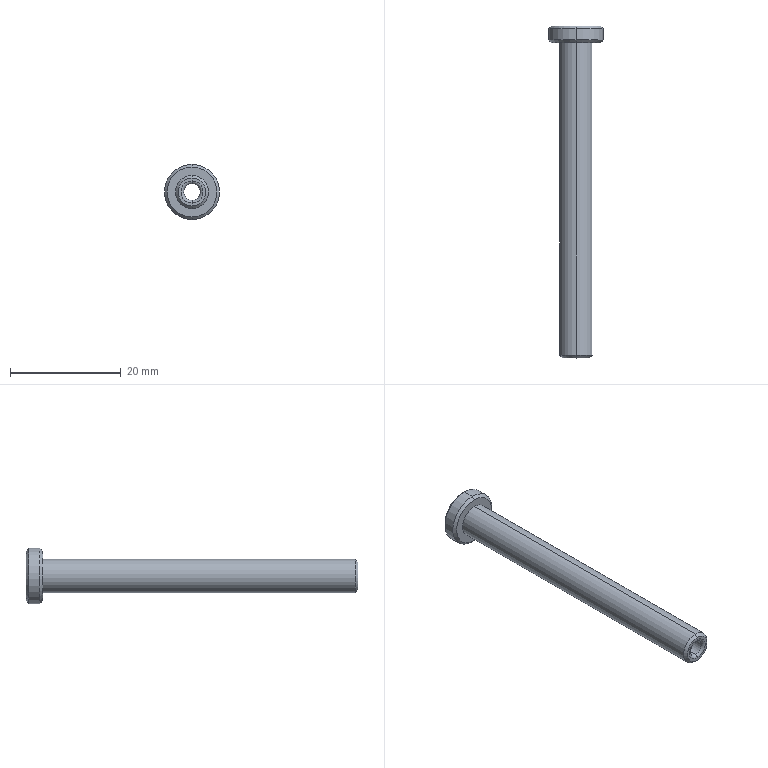Part | SolidWorks | features Chamfer 1, Extrusion 1, Fillet 1, ICE 1 | 1 solid | 19 faces | box 10 x 60 x 10 mm | volume 1412 mm3 | cone 6 | cylinder 6 | torus 4 | plane 3 | commonest cylinder face diameters 3 x2 6 x2 10 x2
STEP:
#1=CARTESIAN_POINT('',(0.,57.,-4.5));
#2=VERTEX_POINT('',#1);
#3=CARTESIAN_POINT('',(0.,57.,4.5));
#4=VERTEX_POINT('',#3);
#5=CARTESIAN_POINT('',(0.,57.,0.));
#6=DIRECTION('',(0.,-1.,0.));
#7=DIRECTION('',(0.,0.,1.));
#8=AXIS2_PLACEMENT_3D('',#5,#6,#7);
#9=CIRCLE('',#8,4.5);
#10=EDGE_CURVE('',#2,#4,#9,.T.);
#11=ORIENTED_EDGE('',*,*,#10,.F.);
#12=CARTESIAN_POINT('',(0.,57.5,-5.));
#13=VERTEX_POINT('',#12);
#14=CARTESIAN_POINT('',(0.,57.5,-5.));
#15=DIRECTION('',(0.,0.7071,-0.7071));
#16=VECTOR('',#15,1000.);
#17=LINE('',#14,#16);
#18=EDGE_CURVE('',#2,#13,#17,.T.);
#19=ORIENTED_EDGE('',*,*,#18,.T.);
#20=CARTESIAN_POINT('',(0.,57.5,5.));
#21=VERTEX_POINT('',#20);
#22=CARTESIAN_POINT('',(0.,57.5,0.));
#23=DIRECTION('',(0.,1.,0.));
#24=DIRECTION('',(0.,0.,1.));
#25=AXIS2_PLACEMENT_3D('',#22,#23,#24);
#26=CIRCLE('',#25,5.);
#27=EDGE_CURVE('',#21,#13,#26,.T.);
#28=ORIENTED_EDGE('',*,*,#27,.F.);
#29=CARTESIAN_POINT('',(0.,57.5,5.));
#30=DIRECTION('',(0.,0.7071,0.7071));
#31=VECTOR('',#30,1000.);
#32=LINE('',#29,#31);
#33=EDGE_CURVE('',#4,#21,#32,.T.);
#34=ORIENTED_EDGE('',*,*,#33,.F.);
#35=EDGE_LOOP('',(#11,#19,#28,#34));
#36=FACE_OUTER_BOUND('',#35,.T.);
#37=CARTESIAN_POINT('',(0.,57.5,0.));
#38=DIRECTION('',(0.,1.,0.));
#39=DIRECTION('',(0.,0.,1.));
#40=AXIS2_PLACEMENT_3D('',#37,#38,#39);
#41=CONICAL_SURFACE('',#40,5.,0.7854);
#42=ADVANCED_FACE('',(#36),#41,.T.);
#43=CARTESIAN_POINT('',(0.,0.,-2.5));
#44=VERTEX_POINT('',#43);
#45=CARTESIAN_POINT('',(0.,0.,2.5));
#46=VERTEX_POINT('',#45);
#47=CARTESIAN_POINT('',(0.,0.,0.));
#48=DIRECTION('',(0.,-1.,0.));
#49=DIRECTION('',(0.,0.,1.));
#50=AXIS2_PLACEMENT_3D('',#47,#48,#49);
#51=CIRCLE('',#50,2.5);
#52=EDGE_CURVE('',#44,#46,#51,.T.);
#53=ORIENTED_EDGE('',*,*,#52,.F.);
#54=CARTESIAN_POINT('',(0.,0.5,-3.));
#55=VERTEX_POINT('',#54);
#56=CARTESIAN_POINT('',(0.,0.5,-3.));
#57=DIRECTION('',(0.,0.7071,-0.7071));
#58=VECTOR('',#57,1000.);
#59=LINE('',#56,#58);
#60=EDGE_CURVE('',#44,#55,#59,.T.);
#61=ORIENTED_EDGE('',*,*,#60,.T.);
#62=CARTESIAN_POINT('',(0.,0.5,3.));
#63=VERTEX_POINT('',#62);
#64=CARTESIAN_POINT('',(0.,0.5,0.));
#65=DIRECTION('',(0.,1.,0.));
#66=DIRECTION('',(0.,0.,1.));
#67=AXIS2_PLACEMENT_3D('',#64,#65,#66);
#68=CIRCLE('',#67,3.);
#69=EDGE_CURVE('',#63,#55,#68,.T.);
#70=ORIENTED_EDGE('',*,*,#69,.F.);
#71=CARTESIAN_POINT('',(0.,0.5,3.));
#72=DIRECTION('',(0.,0.7071,0.7071));
#73=VECTOR('',#72,1000.);
#74=LINE('',#71,#73);
#75=EDGE_CURVE('',#46,#63,#74,.T.);
#76=ORIENTED_EDGE('',*,*,#75,.F.);
#77=EDGE_LOOP('',(#53,#61,#70,#76));
#78=FACE_OUTER_BOUND('',#77,.T.);
#79=CARTESIAN_POINT('',(0.,0.5,0.));
#80=DIRECTION('',(0.,1.,0.));
#81=DIRECTION('',(0.,0.,1.));
#82=AXIS2_PLACEMENT_3D('',#79,#80,#81);
#83=CONICAL_SURFACE('',#82,3.,0.7854);
#84=ADVANCED_FACE('',(#78),#83,.T.);
#85=CARTESIAN_POINT('',(0.,60.,4.5));
#86=VERTEX_POINT('',#85);
#87=CARTESIAN_POINT('',(0.,60.,-4.5));
#88=VERTEX_POINT('',#87);
#89=CARTESIAN_POINT('',(0.,60.,0.));
#90=DIRECTION('',(0.,1.,0.));
#91=DIRECTION('',(0.,0.,1.));
#92=AXIS2_PLACEMENT_3D('',#89,#90,#91);
#93=CIRCLE('',#92,4.5);
#94=EDGE_CURVE('',#86,#88,#93,.T.);
#95=ORIENTED_EDGE('',*,*,#94,.F.);
#96=CARTESIAN_POINT('',(0.,59.5,5.));
#97=VERTEX_POINT('',#96);
#98=CARTESIAN_POINT('',(0.,60.,4.5));
#99=DIRECTION('',(0.,-0.7071,0.7071));
#100=VECTOR('',#99,1000.);
#101=LINE('',#98,#100);
#102=EDGE_CURVE('',#86,#97,#101,.T.);
#103=ORIENTED_EDGE('',*,*,#102,.T.);
#104=CARTESIAN_POINT('',(0.,59.5,-5.));
#105=VERTEX_POINT('',#104);
#106=CARTESIAN_POINT('',(0.,59.5,0.));
#107=DIRECTION('',(0.,-1.,0.));
#108=DIRECTION('',(0.,0.,1.));
#109=AXIS2_PLACEMENT_3D('',#106,#107,#108);
#110=CIRCLE('',#109,5.);
#111=EDGE_CURVE('',#105,#97,#110,.T.);
#112=ORIENTED_EDGE('',*,*,#111,.F.);
#113=CARTESIAN_POINT('',(0.,60.,-4.5));
#114=DIRECTION('',(0.,-0.7071,-0.7071));
#115=VECTOR('',#114,1000.);
#116=LINE('',#113,#115);
#117=EDGE_CURVE('',#88,#105,#116,.T.);
#118=ORIENTED_EDGE('',*,*,#117,.F.);
#119=EDGE_LOOP('',(#95,#103,#112,#118));
#120=FACE_OUTER_BOUND('',#119,.T.);
#121=CARTESIAN_POINT('',(0.,60.,0.));
#122=DIRECTION('',(0.,-1.,0.));
#123=DIRECTION('',(0.,0.,-1.));
#124=AXIS2_PLACEMENT_3D('',#121,#122,#123);
#125=CONICAL_SURFACE('',#124,4.5,0.7854);
#126=ADVANCED_FACE('',(#120),#125,.T.);
#127=CARTESIAN_POINT('',(0.,0.5,-1.5));
#128=VERTEX_POINT('',#127);
#129=CARTESIAN_POINT('',(0.,0.5,1.5));
#130=VERTEX_POINT('',#129);
#131=CARTESIAN_POINT('',(0.,0.5,0.));
#132=DIRECTION('',(0.,-1.,0.));
#133=DIRECTION('',(0.,0.,1.));
#134=AXIS2_PLACEMENT_3D('',#131,#132,#133);
#135=CIRCLE('',#134,1.5);
#136=EDGE_CURVE('',#128,#130,#135,.T.);
#137=ORIENTED_EDGE('',*,*,#136,.F.);
#138=CARTESIAN_POINT('',(0.,0.,-2.));
#139=VERTEX_POINT('',#138);
#140=CARTESIAN_POINT('',(0.,0.5,-2.));
#141=DIRECTION('',(1.,0.,0.));
#142=DIRECTION('',(0.,0.,-1.));
#143=AXIS2_PLACEMENT_3D('',#140,#141,#142);
#144=CIRCLE('',#143,0.5);
#145=EDGE_CURVE('',#128,#139,#144,.T.);
#146=ORIENTED_EDGE('',*,*,#145,.T.);
#147=CARTESIAN_POINT('',(0.,0.,2.));
#148=VERTEX_POINT('',#147);
#149=CARTESIAN_POINT('',(0.,0.,0.));
#150=DIRECTION('',(0.,1.,0.));
#151=DIRECTION('',(0.,0.,1.));
#152=AXIS2_PLACEMENT_3D('',#149,#150,#151);
#153=CIRCLE('',#152,2.);
#154=EDGE_CURVE('',#148,#139,#153,.T.);
#155=ORIENTED_EDGE('',*,*,#154,.F.);
#156=CARTESIAN_POINT('',(0.,0.5,2.));
#157=DIRECTION('',(-1.,0.,0.));
#158=DIRECTION('',(0.,0.,1.));
#159=AXIS2_PLACEMENT_3D('',#156,#157,#158);
#160=CIRCLE('',#159,0.5);
#161=EDGE_CURVE('',#130,#148,#160,.T.);
#162=ORIENTED_EDGE('',*,*,#161,.F.);
#163=EDGE_LOOP('',(#137,#146,#155,#162));
#164=FACE_OUTER_BOUND('',#163,.T.);
#165=CARTESIAN_POINT('',(0.,0.5,0.));
#166=DIRECTION('',(0.,1.,0.));
#167=DIRECTION('',(0.,0.,1.));
#168=AXIS2_PLACEMENT_3D('',#165,#166,#167);
#169=TOROIDAL_SURFACE('',#168,2.,0.5);
#170=ADVANCED_FACE('',(#164),#169,.T.);
#171=CARTESIAN_POINT('',(0.,60.,-2.));
#172=VERTEX_POINT('',#171);
#173=CARTESIAN_POINT('',(0.,60.,2.));
#174=VERTEX_POINT('',#173);
#175=CARTESIAN_POINT('',(0.,60.,0.));
#176=DIRECTION('',(0.,-1.,0.));
#177=DIRECTION('',(0.,0.,1.));
#178=AXIS2_PLACEMENT_3D('',#175,#176,#177);
#179=CIRCLE('',#178,2.);
#180=EDGE_CURVE('',#172,#174,#179,.T.);
#181=ORIENTED_EDGE('',*,*,#180,.F.);
#182=CARTESIAN_POINT('',(0.,59.5,-1.5));
#183=VERTEX_POINT('',#182);
#184=CARTESIAN_POINT('',(0.,59.5,-2.));
#185=DIRECTION('',(1.,0.,0.));
#186=DIRECTION('',(0.,0.,-1.));
#187=AXIS2_PLACEMENT_3D('',#184,#185,#186);
#188=CIRCLE('',#187,0.5);
#189=EDGE_CURVE('',#172,#183,#188,.T.);
#190=ORIENTED_EDGE('',*,*,#189,.T.);
#191=CARTESIAN_POINT('',(0.,59.5,1.5));
#192=VERTEX_POINT('',#191);
#193=CARTESIAN_POINT('',(0.,59.5,0.));
#194=DIRECTION('',(0.,1.,0.));
#195=DIRECTION('',(0.,0.,1.));
#196=AXIS2_PLACEMENT_3D('',#193,#194,#195);
#197=CIRCLE('',#196,1.5);
#198=EDGE_CURVE('',#192,#183,#197,.T.);
#199=ORIENTED_EDGE('',*,*,#198,.F.);
#200=CARTESIAN_POINT('',(0.,59.5,2.));
#201=DIRECTION('',(-1.,0.,0.));
#202=DIRECTION('',(0.,0.,1.));
#203=AXIS2_PLACEMENT_3D('',#200,#201,#202);
#204=CIRCLE('',#203,0.5);
#205=EDGE_CURVE('',#174,#192,#204,.T.);
#206=ORIENTED_EDGE('',*,*,#205,.F.);
#207=EDGE_LOOP('',(#181,#190,#199,#206));
#208=FACE_OUTER_BOUND('',#207,.T.);
#209=CARTESIAN_POINT('',(0.,59.5,0.));
#210=DIRECTION('',(0.,1.,0.));
#211=DIRECTION('',(0.,0.,1.));
#212=AXIS2_PLACEMENT_3D('',#209,#210,#211);
#213=TOROIDAL_SURFACE('',#212,2.,0.5);
#214=ADVANCED_FACE('',(#208),#213,.T.);
#215=ORIENTED_EDGE('',*,*,#27,.T.);
#216=CARTESIAN_POINT('',(0.,57.,-5.));
#217=DIRECTION('',(0.,1.,0.));
#218=VECTOR('',#217,1000.);
#219=LINE('',#216,#218);
#220=EDGE_CURVE('',#13,#105,#219,.T.);
#221=ORIENTED_EDGE('',*,*,#220,.T.);
#222=ORIENTED_EDGE('',*,*,#111,.T.);
#223=CARTESIAN_POINT('',(0.,57.,5.));
#224=DIRECTION('',(0.,1.,0.));
#225=VECTOR('',#224,1000.);
#226=LINE('',#223,#225);
#227=EDGE_CURVE('',#21,#97,#226,.T.);
#228=ORIENTED_EDGE('',*,*,#227,.F.);
#229=EDGE_LOOP('',(#215,#221,#222,#228));
#230=FACE_OUTER_BOUND('',#229,.T.);
#231=CARTESIAN_POINT('',(0.,57.,0.));
#232=DIRECTION('',(0.,1.,0.));
#233=DIRECTION('',(0.,0.,1.));
#234=AXIS2_PLACEMENT_3D('',#231,#232,#233);
#235=CYLINDRICAL_SURFACE('',#234,5.);
#236=ADVANCED_FACE('',(#230),#235,.T.);
#237=CARTESIAN_POINT('',(0.,59.5,0.));
#238=DIRECTION('',(0.,1.,0.));
#239=DIRECTION('',(0.,0.,1.));
#240=AXIS2_PLACEMENT_3D('',#237,#238,#239);
#241=CIRCLE('',#240,1.5);
#242=EDGE_CURVE('',#183,#192,#241,.T.);
#243=ORIENTED_EDGE('',*,*,#242,.T.);
#244=CARTESIAN_POINT('',(0.,60.,1.5));
#245=DIRECTION('',(0.,-1.,0.));
#246=VECTOR('',#245,1000.);
#247=LINE('',#244,#246);
#248=EDGE_CURVE('',#192,#130,#247,.T.);
#249=ORIENTED_EDGE('',*,*,#248,.T.);
#250=CARTESIAN_POINT('',(0.,0.5,0.));
#251=DIRECTION('',(0.,-1.,0.));
#252=DIRECTION('',(0.,0.,1.));
#253=AXIS2_PLACEMENT_3D('',#250,#251,#252);
#254=CIRCLE('',#253,1.5);
#255=EDGE_CURVE('',#130,#128,#254,.T.);
#256=ORIENTED_EDGE('',*,*,#255,.T.);
#257=CARTESIAN_POINT('',(0.,60.,-1.5));
#258=DIRECTION('',(0.,-1.,0.));
#259=VECTOR('',#258,1000.);
#260=LINE('',#257,#259);
#261=EDGE_CURVE('',#183,#128,#260,.T.);
#262=ORIENTED_EDGE('',*,*,#261,.F.);
#263=EDGE_LOOP('',(#243,#249,#256,#262));
#264=FACE_OUTER_BOUND('',#263,.T.);
#265=CARTESIAN_POINT('',(0.,60.,0.));
#266=DIRECTION('',(0.,-1.,0.));
#267=DIRECTION('',(0.,0.,-1.));
#268=AXIS2_PLACEMENT_3D('',#265,#266,#267);
#269=CYLINDRICAL_SURFACE('',#268,1.5);
#270=ADVANCED_FACE('',(#264),#269,.F.);
#271=CARTESIAN_POINT('',(0.,57.,3.));
#272=VERTEX_POINT('',#271);
#273=CARTESIAN_POINT('',(0.,57.,-3.));
#274=VERTEX_POINT('',#273);
#275=CARTESIAN_POINT('',(0.,57.,0.));
#276=DIRECTION('',(0.,1.,0.));
#277=DIRECTION('',(0.,0.,1.));
#278=AXIS2_PLACEMENT_3D('',#275,#276,#277);
#279=CIRCLE('',#278,3.);
#280=EDGE_CURVE('',#272,#274,#279,.T.);
#281=ORIENTED_EDGE('',*,*,#280,.F.);
#282=CARTESIAN_POINT('',(0.,60.,3.));
#283=DIRECTION('',(0.,-1.,0.));
#284=VECTOR('',#283,1000.);
#285=LINE('',#282,#284);
#286=EDGE_CURVE('',#272,#63,#285,.T.);
#287=ORIENTED_EDGE('',*,*,#286,.T.);
#288=ORIENTED_EDGE('',*,*,#69,.T.);
#289=CARTESIAN_POINT('',(0.,60.,-3.));
#290=DIRECTION('',(0.,-1.,0.));
#291=VECTOR('',#290,1000.);
#292=LINE('',#289,#291);
#293=EDGE_CURVE('',#274,#55,#292,.T.);
#294=ORIENTED_EDGE('',*,*,#293,.F.);
#295=EDGE_LOOP('',(#281,#287,#288,#294));
#296=FACE_OUTER_BOUND('',#295,.T.);
#297=CARTESIAN_POINT('',(0.,60.,0.));
#298=DIRECTION('',(0.,-1.,0.));
#299=DIRECTION('',(0.,0.,-1.));
#300=AXIS2_PLACEMENT_3D('',#297,#298,#299);
#301=CYLINDRICAL_SURFACE('',#300,3.);
#302=ADVANCED_FACE('',(#296),#301,.T.);
#303=ORIENTED_EDGE('',*,*,#286,.F.);
#304=CARTESIAN_POINT('',(0.,57.,0.));
#305=DIRECTION('',(0.,1.,0.));
#306=DIRECTION('',(0.,0.,1.));
#307=AXIS2_PLACEMENT_3D('',#304,#305,#306);
#308=CIRCLE('',#307,3.);
#309=EDGE_CURVE('',#274,#272,#308,.T.);
#310=ORIENTED_EDGE('',*,*,#309,.F.);
#311=ORIENTED_EDGE('',*,*,#293,.T.);
#312=CARTESIAN_POINT('',(0.,0.5,0.));
#313=DIRECTION('',(0.,1.,0.));
#314=DIRECTION('',(0.,0.,1.));
#315=AXIS2_PLACEMENT_3D('',#312,#313,#314);
#316=CIRCLE('',#315,3.);
#317=EDGE_CURVE('',#55,#63,#316,.T.);
#318=ORIENTED_EDGE('',*,*,#317,.T.);
#319=EDGE_LOOP('',(#303,#310,#311,#318));
#320=FACE_OUTER_BOUND('',#319,.T.);
#321=CARTESIAN_POINT('',(0.,60.,0.));
#322=DIRECTION('',(0.,-1.,0.));
#323=DIRECTION('',(0.,0.,-1.));
#324=AXIS2_PLACEMENT_3D('',#321,#322,#323);
#325=CYLINDRICAL_SURFACE('',#324,3.);
#326=ADVANCED_FACE('',(#320),#325,.T.);
#327=CARTESIAN_POINT('',(0.,60.,0.));
#328=DIRECTION('',(0.,1.,0.));
#329=DIRECTION('',(0.,0.,1.));
#330=AXIS2_PLACEMENT_3D('',#327,#328,#329);
#331=CIRCLE('',#330,4.5);
#332=EDGE_CURVE('',#88,#86,#331,.T.);
#333=ORIENTED_EDGE('',*,*,#332,.T.);
#334=ORIENTED_EDGE('',*,*,#94,.T.);
#335=EDGE_LOOP('',(#333,#334));
#336=FACE_OUTER_BOUND('',#335,.T.);
#337=CARTESIAN_POINT('',(0.,60.,0.));
#338=DIRECTION('',(0.,-1.,0.));
#339=DIRECTION('',(0.,0.,1.));
#340=AXIS2_PLACEMENT_3D('',#337,#338,#339);
#341=CIRCLE('',#340,2.);
#342=EDGE_CURVE('',#174,#172,#341,.T.);
#343=ORIENTED_EDGE('',*,*,#342,.T.);
#344=ORIENTED_EDGE('',*,*,#180,.T.);
#345=EDGE_LOOP('',(#343,#344));
#346=FACE_BOUND('',#345,.T.);
#347=CARTESIAN_POINT('',(0.,60.,0.));
#348=DIRECTION('',(0.,1.,0.));
#349=DIRECTION('',(0.,0.,1.));
#350=AXIS2_PLACEMENT_3D('',#347,#348,#349);
#351=PLANE('',#350);
#352=ADVANCED_FACE('',(#336,#346),#351,.T.);
#353=CARTESIAN_POINT('',(0.,0.,0.));
#354=DIRECTION('',(0.,-1.,0.));
#355=DIRECTION('',(0.,0.,1.));
#356=AXIS2_PLACEMENT_3D('',#353,#354,#355);
#357=CIRCLE('',#356,2.5);
#358=EDGE_CURVE('',#46,#44,#357,.T.);
#359=ORIENTED_EDGE('',*,*,#358,.T.);
#360=ORIENTED_EDGE('',*,*,#52,.T.);
#361=EDGE_LOOP('',(#359,#360));
#362=FACE_OUTER_BOUND('',#361,.T.);
#363=ORIENTED_EDGE('',*,*,#154,.T.);
#364=CARTESIAN_POINT('',(0.,0.,0.));
#365=DIRECTION('',(0.,1.,0.));
#366=DIRECTION('',(0.,0.,1.));
#367=AXIS2_PLACEMENT_3D('',#364,#365,#366);
#368=CIRCLE('',#367,2.);
#369=EDGE_CURVE('',#139,#148,#368,.T.);
#370=ORIENTED_EDGE('',*,*,#369,.T.);
#371=EDGE_LOOP('',(#363,#370));
#372=FACE_BOUND('',#371,.T.);
#373=CARTESIAN_POINT('',(0.,0.,0.));
#374=DIRECTION('',(0.,1.,0.));
#375=DIRECTION('',(0.,0.,1.));
#376=AXIS2_PLACEMENT_3D('',#373,#374,#375);
#377=PLANE('',#376);
#378=ADVANCED_FACE('',(#362,#372),#377,.F.);
#379=ORIENTED_EDGE('',*,*,#248,.F.);
#380=ORIENTED_EDGE('',*,*,#198,.T.);
#381=ORIENTED_EDGE('',*,*,#261,.T.);
#382=ORIENTED_EDGE('',*,*,#136,.T.);
#383=EDGE_LOOP('',(#379,#380,#381,#382));
#384=FACE_OUTER_BOUND('',#383,.T.);
#385=CARTESIAN_POINT('',(0.,60.,0.));
#386=DIRECTION('',(0.,-1.,0.));
#387=DIRECTION('',(0.,0.,-1.));
#388=AXIS2_PLACEMENT_3D('',#385,#386,#387);
#389=CYLINDRICAL_SURFACE('',#388,1.5);
#390=ADVANCED_FACE('',(#384),#389,.F.);
#391=CARTESIAN_POINT('',(0.,57.,0.));
#392=DIRECTION('',(0.,-1.,0.));
#393=DIRECTION('',(0.,0.,1.));
#394=AXIS2_PLACEMENT_3D('',#391,#392,#393);
#395=CIRCLE('',#394,4.5);
#396=EDGE_CURVE('',#4,#2,#395,.T.);
#397=ORIENTED_EDGE('',*,*,#396,.T.);
#398=ORIENTED_EDGE('',*,*,#10,.T.);
#399=EDGE_LOOP('',(#397,#398));
#400=FACE_OUTER_BOUND('',#399,.T.);
#401=ORIENTED_EDGE('',*,*,#309,.T.);
#402=ORIENTED_EDGE('',*,*,#280,.T.);
#403=EDGE_LOOP('',(#401,#402));
#404=FACE_BOUND('',#403,.T.);
#405=CARTESIAN_POINT('',(0.,57.,0.));
#406=DIRECTION('',(0.,1.,0.));
#407=DIRECTION('',(0.,0.,1.));
#408=AXIS2_PLACEMENT_3D('',#405,#406,#407);
#409=PLANE('',#408);
#410=ADVANCED_FACE('',(#400,#404),#409,.F.);
#411=ORIENTED_EDGE('',*,*,#220,.F.);
#412=CARTESIAN_POINT('',(0.,57.5,0.));
#413=DIRECTION('',(0.,1.,0.));
#414=DIRECTION('',(0.,0.,1.));
#415=AXIS2_PLACEMENT_3D('',#412,#413,#414);
#416=CIRCLE('',#415,5.);
#417=EDGE_CURVE('',#13,#21,#416,.T.);
#418=ORIENTED_EDGE('',*,*,#417,.T.);
#419=ORIENTED_EDGE('',*,*,#227,.T.);
#420=CARTESIAN_POINT('',(0.,59.5,0.));
#421=DIRECTION('',(0.,-1.,0.));
#422=DIRECTION('',(0.,0.,1.));
#423=AXIS2_PLACEMENT_3D('',#420,#421,#422);
#424=CIRCLE('',#423,5.);
#425=EDGE_CURVE('',#97,#105,#424,.T.);
#426=ORIENTED_EDGE('',*,*,#425,.T.);
#427=EDGE_LOOP('',(#411,#418,#419,#426));
#428=FACE_OUTER_BOUND('',#427,.T.);
#429=CARTESIAN_POINT('',(0.,57.,0.));
#430=DIRECTION('',(0.,1.,0.));
#431=DIRECTION('',(0.,0.,1.));
#432=AXIS2_PLACEMENT_3D('',#429,#430,#431);
#433=CYLINDRICAL_SURFACE('',#432,5.);
#434=ADVANCED_FACE('',(#428),#433,.T.);
#435=ORIENTED_EDGE('',*,*,#189,.F.);
#436=ORIENTED_EDGE('',*,*,#342,.F.);
#437=ORIENTED_EDGE('',*,*,#205,.T.);
#438=ORIENTED_EDGE('',*,*,#242,.F.);
#439=EDGE_LOOP('',(#435,#436,#437,#438));
#440=FACE_OUTER_BOUND('',#439,.T.);
#441=CARTESIAN_POINT('',(0.,59.5,0.));
#442=DIRECTION('',(0.,1.,0.));
#443=DIRECTION('',(0.,0.,1.));
#444=AXIS2_PLACEMENT_3D('',#441,#442,#443);
#445=TOROIDAL_SURFACE('',#444,2.,0.5);
#446=ADVANCED_FACE('',(#440),#445,.T.);
#447=ORIENTED_EDGE('',*,*,#145,.F.);
#448=ORIENTED_EDGE('',*,*,#255,.F.);
#449=ORIENTED_EDGE('',*,*,#161,.T.);
#450=ORIENTED_EDGE('',*,*,#369,.F.);
#451=EDGE_LOOP('',(#447,#448,#449,#450));
#452=FACE_OUTER_BOUND('',#451,.T.);
#453=CARTESIAN_POINT('',(0.,0.5,0.));
#454=DIRECTION('',(0.,1.,0.));
#455=DIRECTION('',(0.,0.,1.));
#456=AXIS2_PLACEMENT_3D('',#453,#454,#455);
#457=TOROIDAL_SURFACE('',#456,2.,0.5);
#458=ADVANCED_FACE('',(#452),#457,.T.);
#459=ORIENTED_EDGE('',*,*,#102,.F.);
#460=ORIENTED_EDGE('',*,*,#332,.F.);
#461=ORIENTED_EDGE('',*,*,#117,.T.);
#462=ORIENTED_EDGE('',*,*,#425,.F.);
#463=EDGE_LOOP('',(#459,#460,#461,#462));
#464=FACE_OUTER_BOUND('',#463,.T.);
#465=CARTESIAN_POINT('',(0.,60.,0.));
#466=DIRECTION('',(0.,-1.,0.));
#467=DIRECTION('',(0.,0.,-1.));
#468=AXIS2_PLACEMENT_3D('',#465,#466,#467);
#469=CONICAL_SURFACE('',#468,4.5,0.7854);
#470=ADVANCED_FACE('',(#464),#469,.T.);
#471=ORIENTED_EDGE('',*,*,#60,.F.);
#472=ORIENTED_EDGE('',*,*,#358,.F.);
#473=ORIENTED_EDGE('',*,*,#75,.T.);
#474=ORIENTED_EDGE('',*,*,#317,.F.);
#475=EDGE_LOOP('',(#471,#472,#473,#474));
#476=FACE_OUTER_BOUND('',#475,.T.);
#477=CARTESIAN_POINT('',(0.,0.5,0.));
#478=DIRECTION('',(0.,1.,0.));
#479=DIRECTION('',(0.,0.,1.));
#480=AXIS2_PLACEMENT_3D('',#477,#478,#479);
#481=CONICAL_SURFACE('',#480,3.,0.7854);
#482=ADVANCED_FACE('',(#476),#481,.T.);
#483=ORIENTED_EDGE('',*,*,#18,.F.);
#484=ORIENTED_EDGE('',*,*,#396,.F.);
#485=ORIENTED_EDGE('',*,*,#33,.T.);
#486=ORIENTED_EDGE('',*,*,#417,.F.);
#487=EDGE_LOOP('',(#483,#484,#485,#486));
#488=FACE_OUTER_BOUND('',#487,.T.);
#489=CARTESIAN_POINT('',(0.,57.5,0.));
#490=DIRECTION('',(0.,1.,0.));
#491=DIRECTION('',(0.,0.,1.));
#492=AXIS2_PLACEMENT_3D('',#489,#490,#491);
#493=CONICAL_SURFACE('',#492,5.,0.7854);
#494=ADVANCED_FACE('',(#488),#493,.T.);
#495=CLOSED_SHELL('',(#42,#84,#126,#170,#214,#236,#270,#302,#326,#352,#378,#390,#410,#434,#446,#458,#470,#482,#494));
#496=MANIFOLD_SOLID_BREP('',#495);
#497=CARTESIAN_POINT('',(0.,0.,0.));
#498=DIRECTION('',(0.,0.,1.));
#499=DIRECTION('',(1.,0.,0.));
#500=AXIS2_PLACEMENT_3D('',#497,#498,#499);
#501=(LENGTH_UNIT()NAMED_UNIT(*)SI_UNIT(.MILLI.,.METRE.));
#502=UNCERTAINTY_MEASURE_WITH_UNIT(LENGTH_MEASURE(0.00001),#501,'','');
#503=(NAMED_UNIT(*)PLANE_ANGLE_UNIT()SI_UNIT($,.RADIAN.));
#504=(NAMED_UNIT(*)SI_UNIT($,.STERADIAN.)SOLID_ANGLE_UNIT());
#505=(GEOMETRIC_REPRESENTATION_CONTEXT(3)GLOBAL_UNCERTAINTY_ASSIGNED_CONTEXT((#502))GLOBAL_UNIT_ASSIGNED_CONTEXT((#501,#503,#504))REPRESENTATION_CONTEXT('',''));
#506=ADVANCED_BREP_SHAPE_REPRESENTATION('',(#496,#500),#505);